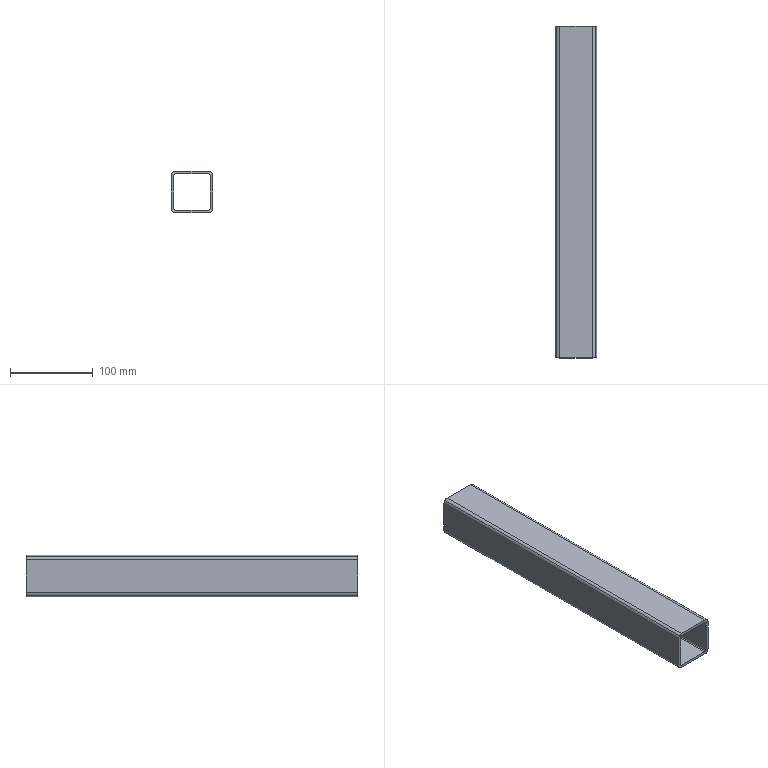Part | STEP file | POST.SQ.PIPE.11.stp | 1 solid | 26 faces | box 50 x 400 x 50 mm | volume 231705 mm3 | cylinder 16 | plane 10 | commonest cylinder face diameters 4 x8 10.4 x8